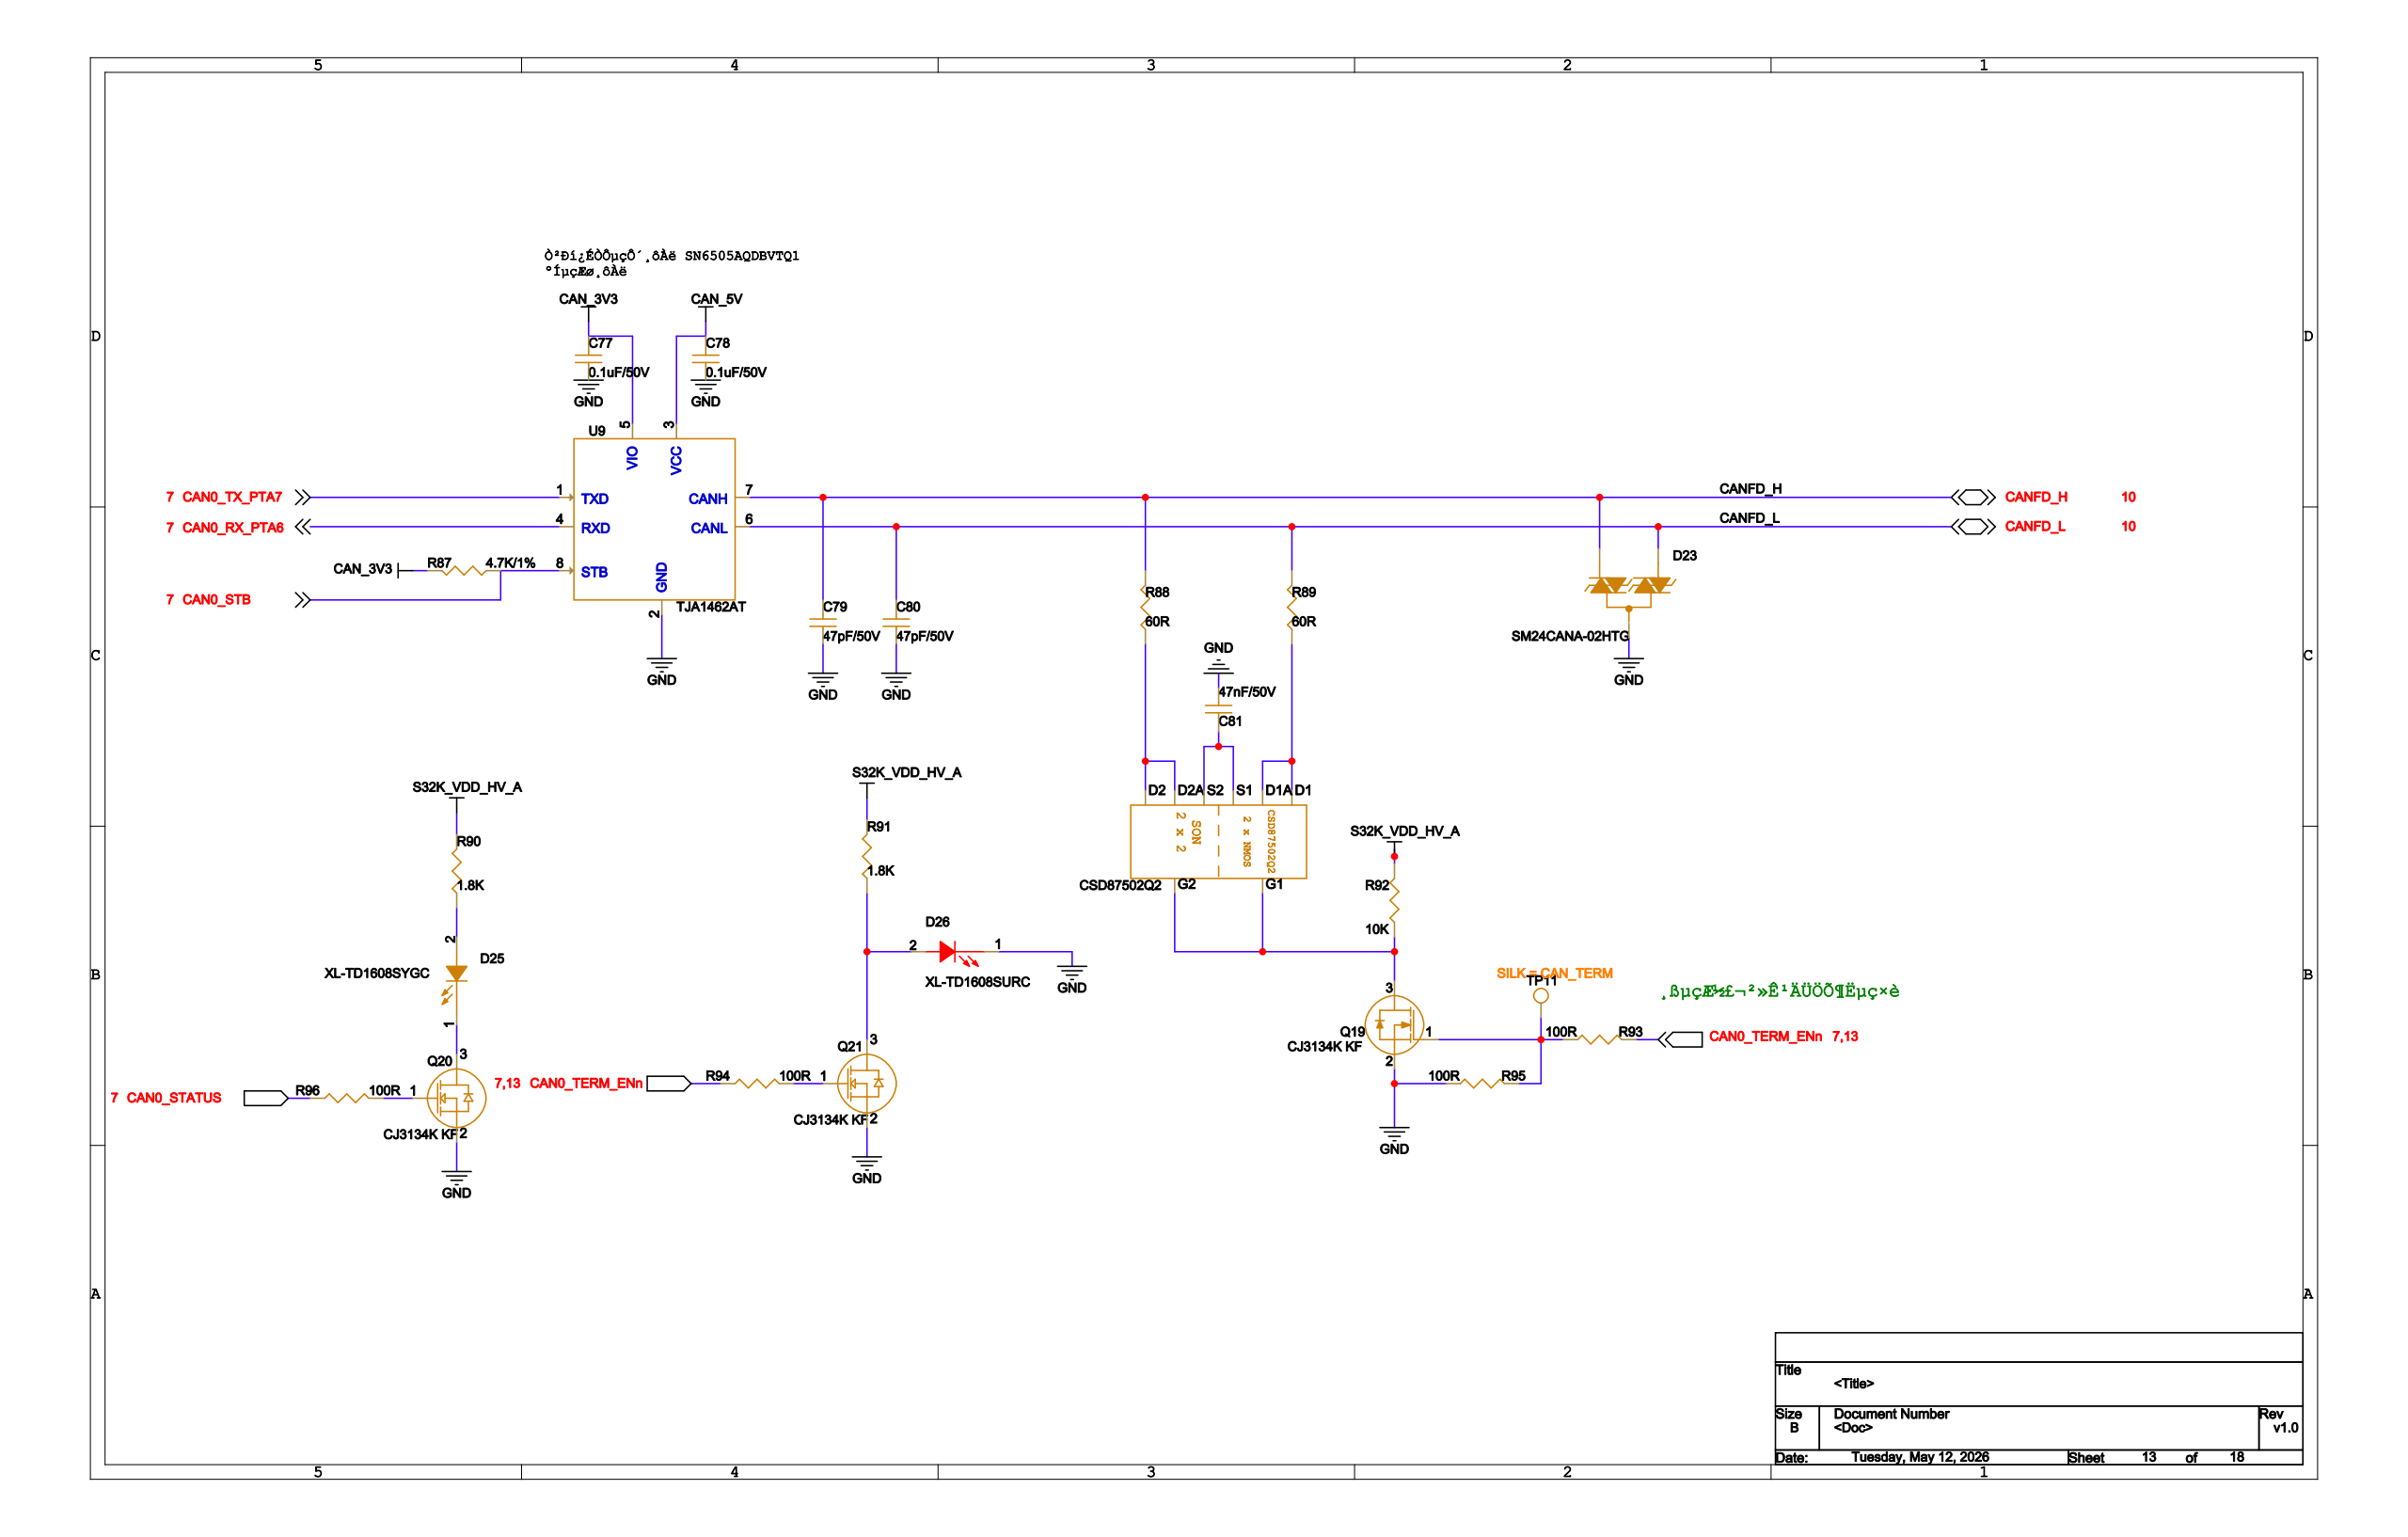Circuit board | Cadence Allegro | 330 parts | 215 nets | one sheet of the schematic
Parts on this sheet (reference | value | footprint):
C77 | 0.1uF/50V | C0402
C78 | 0.1uF/50V | C0402
C79 | 47pF/50V | C0402
C80 | 47pF/50V | C0402
C81 | 47nF/50V | C0402
D23 | SM24CANA-02HTG | SOT23-3
D25 | XL-TD1608SYGC | LED0603
D26 | XL-TD1608SURC | LED0603
Q19 | CJ3134K KF | SOT723
Q20 | CJ3134K KF | SOT-723
Q21 | CJ3134K KF | SOT-723
R87 | 4.7K/1% | R0402
R88 | 60R | R0402
R89 | 60R | R0402
R90 | 1.8K | 0402
R91 | 1.8K | 0402
R92 | 10K | 0402
R93 | 100R | 0402
R94 | 100R | 0402
R95 | 100R | 0402
R96 | 100R | 0402
TP11 | TP | S0400CI
U9 | TJA1462AT | SO8
Nets of these parts (net: part-pin ...):
CANFD_H: C79-2 D23-2 R88-1 U9-7
CANFD_L: C80-2 D23-1 R89-1 U9-6
GND: C77-1 C78-1 C79-1 C80-1 C81-1 D23-3 D26-1 Q19-2 Q20-2 Q21-2 R95-2 U9-2
CAN_3V3: C77-2 R87-1 U9-5
CAN0_STB: R87-2 U9-8
N16956770: R88-2
N16956772: R89-2
S32K_VDD_HV_A: R90-2 R91-2 R92-2
CAN_5V: C78-2 U9-3
N16956774: C81-2
N16960584: D26-2 Q21-3 R91-1
N16959157: D25-1 Q20-3
N16959143: D25-2 R90-1
N16959183: Q20-1 R96-2
N16960633: Q21-1 R94-2
N16956625: Q19-3 R92-1
CAN0_RX_PTA6: U9-4
CAN0_TX_PTA7: U9-1
CAN0_TERM_ENN: R93-1 R94-1
CAN0_STATUS: R96-1
N16956660: Q19-1 R93-2 R95-1 TP11-1